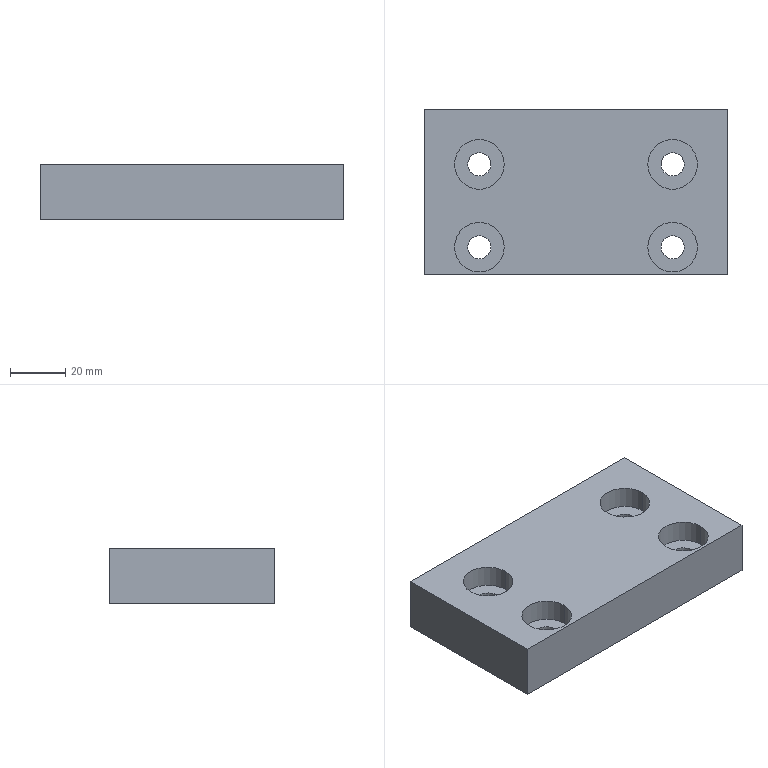Part | SolidWorks | features BaseBody 1 | 1 solid | 34 faces | box 110 x 60 x 20 mm | volume 118905 mm3 | cylinder 20 | plane 10 | cone 4 | commonest cylinder face diameters 8.4 x8 18 x8 10.2 x4
STEP:
#1=CARTESIAN_POINT('',(185.8,110.,-32.879));
#2=VERTEX_POINT('',#1);
#3=CARTESIAN_POINT('',(194.2,110.,-32.879));
#4=VERTEX_POINT('',#3);
#5=CARTESIAN_POINT('',(190.,110.,-32.879));
#6=DIRECTION('',(0.,0.,1.));
#7=DIRECTION('',(1.,0.,0.));
#8=AXIS2_PLACEMENT_3D('',#5,#6,#7);
#9=CIRCLE('',#8,4.2);
#10=EDGE_CURVE('',#2,#4,#9,.T.);
#11=ORIENTED_EDGE('',*,*,#10,.F.);
#12=CARTESIAN_POINT('',(185.8,110.,-20.879));
#13=VERTEX_POINT('',#12);
#14=CARTESIAN_POINT('',(185.8,110.,-12.879));
#15=DIRECTION('',(0.,0.,1.));
#16=VECTOR('',#15,1000.);
#17=LINE('',#14,#16);
#18=EDGE_CURVE('',#2,#13,#17,.T.);
#19=ORIENTED_EDGE('',*,*,#18,.T.);
#20=CARTESIAN_POINT('',(194.2,110.,-20.879));
#21=VERTEX_POINT('',#20);
#22=CARTESIAN_POINT('',(190.,110.,-20.879));
#23=DIRECTION('',(0.,0.,-1.));
#24=DIRECTION('',(1.,0.,0.));
#25=AXIS2_PLACEMENT_3D('',#22,#23,#24);
#26=CIRCLE('',#25,4.2);
#27=EDGE_CURVE('',#21,#13,#26,.T.);
#28=ORIENTED_EDGE('',*,*,#27,.F.);
#29=CARTESIAN_POINT('',(194.2,110.,-12.879));
#30=DIRECTION('',(0.,0.,1.));
#31=VECTOR('',#30,1000.);
#32=LINE('',#29,#31);
#33=EDGE_CURVE('',#4,#21,#32,.T.);
#34=ORIENTED_EDGE('',*,*,#33,.F.);
#35=EDGE_LOOP('',(#11,#19,#28,#34));
#36=FACE_OUTER_BOUND('',#35,.T.);
#37=CARTESIAN_POINT('',(190.,110.,-12.879));
#38=DIRECTION('',(0.,0.,1.));
#39=DIRECTION('',(1.,0.,0.));
#40=AXIS2_PLACEMENT_3D('',#37,#38,#39);
#41=CYLINDRICAL_SURFACE('',#40,4.2);
#42=ADVANCED_FACE('',(#36),#41,.F.);
#43=CARTESIAN_POINT('',(185.8,80.,-32.879));
#44=VERTEX_POINT('',#43);
#45=CARTESIAN_POINT('',(194.2,80.,-32.879));
#46=VERTEX_POINT('',#45);
#47=CARTESIAN_POINT('',(190.,80.,-32.879));
#48=DIRECTION('',(0.,0.,1.));
#49=DIRECTION('',(1.,0.,0.));
#50=AXIS2_PLACEMENT_3D('',#47,#48,#49);
#51=CIRCLE('',#50,4.2);
#52=EDGE_CURVE('',#44,#46,#51,.T.);
#53=ORIENTED_EDGE('',*,*,#52,.F.);
#54=CARTESIAN_POINT('',(185.8,80.,-20.879));
#55=VERTEX_POINT('',#54);
#56=CARTESIAN_POINT('',(185.8,80.,-12.879));
#57=DIRECTION('',(0.,0.,1.));
#58=VECTOR('',#57,1000.);
#59=LINE('',#56,#58);
#60=EDGE_CURVE('',#44,#55,#59,.T.);
#61=ORIENTED_EDGE('',*,*,#60,.T.);
#62=CARTESIAN_POINT('',(194.2,80.,-20.879));
#63=VERTEX_POINT('',#62);
#64=CARTESIAN_POINT('',(190.,80.,-20.879));
#65=DIRECTION('',(0.,0.,-1.));
#66=DIRECTION('',(1.,0.,0.));
#67=AXIS2_PLACEMENT_3D('',#64,#65,#66);
#68=CIRCLE('',#67,4.2);
#69=EDGE_CURVE('',#63,#55,#68,.T.);
#70=ORIENTED_EDGE('',*,*,#69,.F.);
#71=CARTESIAN_POINT('',(194.2,80.,-12.879));
#72=DIRECTION('',(0.,0.,1.));
#73=VECTOR('',#72,1000.);
#74=LINE('',#71,#73);
#75=EDGE_CURVE('',#46,#63,#74,.T.);
#76=ORIENTED_EDGE('',*,*,#75,.F.);
#77=EDGE_LOOP('',(#53,#61,#70,#76));
#78=FACE_OUTER_BOUND('',#77,.T.);
#79=CARTESIAN_POINT('',(190.,80.,-12.879));
#80=DIRECTION('',(0.,0.,1.));
#81=DIRECTION('',(1.,0.,0.));
#82=AXIS2_PLACEMENT_3D('',#79,#80,#81);
#83=CYLINDRICAL_SURFACE('',#82,4.2);
#84=ADVANCED_FACE('',(#78),#83,.F.);
#85=CARTESIAN_POINT('',(255.8,80.,-32.879));
#86=VERTEX_POINT('',#85);
#87=CARTESIAN_POINT('',(264.2,80.,-32.879));
#88=VERTEX_POINT('',#87);
#89=CARTESIAN_POINT('',(260.,80.,-32.879));
#90=DIRECTION('',(0.,0.,1.));
#91=DIRECTION('',(1.,0.,0.));
#92=AXIS2_PLACEMENT_3D('',#89,#90,#91);
#93=CIRCLE('',#92,4.2);
#94=EDGE_CURVE('',#86,#88,#93,.T.);
#95=ORIENTED_EDGE('',*,*,#94,.F.);
#96=CARTESIAN_POINT('',(255.8,80.,-20.879));
#97=VERTEX_POINT('',#96);
#98=CARTESIAN_POINT('',(255.8,80.,-12.879));
#99=DIRECTION('',(0.,0.,1.));
#100=VECTOR('',#99,1000.);
#101=LINE('',#98,#100);
#102=EDGE_CURVE('',#86,#97,#101,.T.);
#103=ORIENTED_EDGE('',*,*,#102,.T.);
#104=CARTESIAN_POINT('',(264.2,80.,-20.879));
#105=VERTEX_POINT('',#104);
#106=CARTESIAN_POINT('',(260.,80.,-20.879));
#107=DIRECTION('',(0.,0.,-1.));
#108=DIRECTION('',(1.,0.,0.));
#109=AXIS2_PLACEMENT_3D('',#106,#107,#108);
#110=CIRCLE('',#109,4.2);
#111=EDGE_CURVE('',#105,#97,#110,.T.);
#112=ORIENTED_EDGE('',*,*,#111,.F.);
#113=CARTESIAN_POINT('',(264.2,80.,-12.879));
#114=DIRECTION('',(0.,0.,1.));
#115=VECTOR('',#114,1000.);
#116=LINE('',#113,#115);
#117=EDGE_CURVE('',#88,#105,#116,.T.);
#118=ORIENTED_EDGE('',*,*,#117,.F.);
#119=EDGE_LOOP('',(#95,#103,#112,#118));
#120=FACE_OUTER_BOUND('',#119,.T.);
#121=CARTESIAN_POINT('',(260.,80.,-12.879));
#122=DIRECTION('',(0.,0.,1.));
#123=DIRECTION('',(1.,0.,0.));
#124=AXIS2_PLACEMENT_3D('',#121,#122,#123);
#125=CYLINDRICAL_SURFACE('',#124,4.2);
#126=ADVANCED_FACE('',(#120),#125,.F.);
#127=CARTESIAN_POINT('',(255.8,110.,-32.879));
#128=VERTEX_POINT('',#127);
#129=CARTESIAN_POINT('',(264.2,110.,-32.879));
#130=VERTEX_POINT('',#129);
#131=CARTESIAN_POINT('',(260.,110.,-32.879));
#132=DIRECTION('',(0.,0.,1.));
#133=DIRECTION('',(1.,0.,0.));
#134=AXIS2_PLACEMENT_3D('',#131,#132,#133);
#135=CIRCLE('',#134,4.2);
#136=EDGE_CURVE('',#128,#130,#135,.T.);
#137=ORIENTED_EDGE('',*,*,#136,.F.);
#138=CARTESIAN_POINT('',(255.8,110.,-20.879));
#139=VERTEX_POINT('',#138);
#140=CARTESIAN_POINT('',(255.8,110.,-12.879));
#141=DIRECTION('',(0.,0.,1.));
#142=VECTOR('',#141,1000.);
#143=LINE('',#140,#142);
#144=EDGE_CURVE('',#128,#139,#143,.T.);
#145=ORIENTED_EDGE('',*,*,#144,.T.);
#146=CARTESIAN_POINT('',(264.2,110.,-20.879));
#147=VERTEX_POINT('',#146);
#148=CARTESIAN_POINT('',(260.,110.,-20.879));
#149=DIRECTION('',(0.,0.,-1.));
#150=DIRECTION('',(1.,0.,0.));
#151=AXIS2_PLACEMENT_3D('',#148,#149,#150);
#152=CIRCLE('',#151,4.2);
#153=EDGE_CURVE('',#147,#139,#152,.T.);
#154=ORIENTED_EDGE('',*,*,#153,.F.);
#155=CARTESIAN_POINT('',(264.2,110.,-12.879));
#156=DIRECTION('',(0.,0.,1.));
#157=VECTOR('',#156,1000.);
#158=LINE('',#155,#157);
#159=EDGE_CURVE('',#130,#147,#158,.T.);
#160=ORIENTED_EDGE('',*,*,#159,.F.);
#161=EDGE_LOOP('',(#137,#145,#154,#160));
#162=FACE_OUTER_BOUND('',#161,.T.);
#163=CARTESIAN_POINT('',(260.,110.,-12.879));
#164=DIRECTION('',(0.,0.,1.));
#165=DIRECTION('',(1.,0.,0.));
#166=AXIS2_PLACEMENT_3D('',#163,#164,#165);
#167=CYLINDRICAL_SURFACE('',#166,4.2);
#168=ADVANCED_FACE('',(#162),#167,.F.);
#169=CARTESIAN_POINT('',(272.,117.,-27.979));
#170=VERTEX_POINT('',#169);
#171=CARTESIAN_POINT('',(272.,117.,-17.779));
#172=VERTEX_POINT('',#171);
#173=CARTESIAN_POINT('',(272.,117.,-22.879));
#174=DIRECTION('',(0.,1.,0.));
#175=DIRECTION('',(0.,0.,1.));
#176=AXIS2_PLACEMENT_3D('',#173,#174,#175);
#177=CIRCLE('',#176,5.1);
#178=EDGE_CURVE('',#170,#172,#177,.T.);
#179=ORIENTED_EDGE('',*,*,#178,.F.);
#180=CARTESIAN_POINT('',(272.,130.,-27.979));
#181=VERTEX_POINT('',#180);
#182=CARTESIAN_POINT('',(272.,130.,-27.979));
#183=DIRECTION('',(0.,1.,0.));
#184=VECTOR('',#183,1000.);
#185=LINE('',#182,#184);
#186=EDGE_CURVE('',#170,#181,#185,.T.);
#187=ORIENTED_EDGE('',*,*,#186,.T.);
#188=CARTESIAN_POINT('',(272.,130.,-17.779));
#189=VERTEX_POINT('',#188);
#190=CARTESIAN_POINT('',(272.,130.,-22.879));
#191=DIRECTION('',(0.,1.,0.));
#192=DIRECTION('',(0.,0.,1.));
#193=AXIS2_PLACEMENT_3D('',#190,#191,#192);
#194=CIRCLE('',#193,5.1);
#195=EDGE_CURVE('',#181,#189,#194,.T.);
#196=ORIENTED_EDGE('',*,*,#195,.T.);
#197=CARTESIAN_POINT('',(272.,130.,-17.779));
#198=DIRECTION('',(0.,1.,0.));
#199=VECTOR('',#198,1000.);
#200=LINE('',#197,#199);
#201=EDGE_CURVE('',#172,#189,#200,.T.);
#202=ORIENTED_EDGE('',*,*,#201,.F.);
#203=EDGE_LOOP('',(#179,#187,#196,#202));
#204=FACE_OUTER_BOUND('',#203,.T.);
#205=CARTESIAN_POINT('',(272.,130.,-22.879));
#206=DIRECTION('',(0.,1.,0.));
#207=DIRECTION('',(0.,0.,1.));
#208=AXIS2_PLACEMENT_3D('',#205,#206,#207);
#209=CYLINDRICAL_SURFACE('',#208,5.1);
#210=ADVANCED_FACE('',(#204),#209,.F.);
#211=CARTESIAN_POINT('',(178.,117.,-27.979));
#212=VERTEX_POINT('',#211);
#213=CARTESIAN_POINT('',(178.,117.,-17.779));
#214=VERTEX_POINT('',#213);
#215=CARTESIAN_POINT('',(178.,117.,-22.879));
#216=DIRECTION('',(0.,1.,0.));
#217=DIRECTION('',(0.,0.,1.));
#218=AXIS2_PLACEMENT_3D('',#215,#216,#217);
#219=CIRCLE('',#218,5.1);
#220=EDGE_CURVE('',#212,#214,#219,.T.);
#221=ORIENTED_EDGE('',*,*,#220,.F.);
#222=CARTESIAN_POINT('',(178.,130.,-27.979));
#223=VERTEX_POINT('',#222);
#224=CARTESIAN_POINT('',(178.,130.,-27.979));
#225=DIRECTION('',(0.,1.,0.));
#226=VECTOR('',#225,1000.);
#227=LINE('',#224,#226);
#228=EDGE_CURVE('',#212,#223,#227,.T.);
#229=ORIENTED_EDGE('',*,*,#228,.T.);
#230=CARTESIAN_POINT('',(178.,130.,-17.779));
#231=VERTEX_POINT('',#230);
#232=CARTESIAN_POINT('',(178.,130.,-22.879));
#233=DIRECTION('',(0.,1.,0.));
#234=DIRECTION('',(0.,0.,1.));
#235=AXIS2_PLACEMENT_3D('',#232,#233,#234);
#236=CIRCLE('',#235,5.1);
#237=EDGE_CURVE('',#223,#231,#236,.T.);
#238=ORIENTED_EDGE('',*,*,#237,.T.);
#239=CARTESIAN_POINT('',(178.,130.,-17.779));
#240=DIRECTION('',(0.,1.,0.));
#241=VECTOR('',#240,1000.);
#242=LINE('',#239,#241);
#243=EDGE_CURVE('',#214,#231,#242,.T.);
#244=ORIENTED_EDGE('',*,*,#243,.F.);
#245=EDGE_LOOP('',(#221,#229,#238,#244));
#246=FACE_OUTER_BOUND('',#245,.T.);
#247=CARTESIAN_POINT('',(178.,130.,-22.879));
#248=DIRECTION('',(0.,1.,0.));
#249=DIRECTION('',(0.,0.,1.));
#250=AXIS2_PLACEMENT_3D('',#247,#248,#249);
#251=CYLINDRICAL_SURFACE('',#250,5.1);
#252=ADVANCED_FACE('',(#246),#251,.F.);
#253=CARTESIAN_POINT('',(199.,110.,-20.879));
#254=VERTEX_POINT('',#253);
#255=CARTESIAN_POINT('',(181.,110.,-20.879));
#256=VERTEX_POINT('',#255);
#257=CARTESIAN_POINT('',(190.,110.,-20.879));
#258=DIRECTION('',(0.,0.,-1.));
#259=DIRECTION('',(1.,0.,0.));
#260=AXIS2_PLACEMENT_3D('',#257,#258,#259);
#261=CIRCLE('',#260,9.);
#262=EDGE_CURVE('',#254,#256,#261,.T.);
#263=ORIENTED_EDGE('',*,*,#262,.T.);
#264=CARTESIAN_POINT('',(181.,110.,-12.879));
#265=VERTEX_POINT('',#264);
#266=CARTESIAN_POINT('',(181.,110.,-12.879));
#267=DIRECTION('',(0.,0.,1.));
#268=VECTOR('',#267,1000.);
#269=LINE('',#266,#268);
#270=EDGE_CURVE('',#256,#265,#269,.T.);
#271=ORIENTED_EDGE('',*,*,#270,.T.);
#272=CARTESIAN_POINT('',(199.,110.,-12.879));
#273=VERTEX_POINT('',#272);
#274=CARTESIAN_POINT('',(190.,110.,-12.879));
#275=DIRECTION('',(0.,0.,1.));
#276=DIRECTION('',(1.,0.,0.));
#277=AXIS2_PLACEMENT_3D('',#274,#275,#276);
#278=CIRCLE('',#277,9.);
#279=EDGE_CURVE('',#265,#273,#278,.T.);
#280=ORIENTED_EDGE('',*,*,#279,.T.);
#281=CARTESIAN_POINT('',(199.,110.,-12.879));
#282=DIRECTION('',(0.,0.,1.));
#283=VECTOR('',#282,1000.);
#284=LINE('',#281,#283);
#285=EDGE_CURVE('',#254,#273,#284,.T.);
#286=ORIENTED_EDGE('',*,*,#285,.F.);
#287=EDGE_LOOP('',(#263,#271,#280,#286));
#288=FACE_OUTER_BOUND('',#287,.T.);
#289=CARTESIAN_POINT('',(190.,110.,-12.879));
#290=DIRECTION('',(0.,0.,1.));
#291=DIRECTION('',(1.,0.,0.));
#292=AXIS2_PLACEMENT_3D('',#289,#290,#291);
#293=CYLINDRICAL_SURFACE('',#292,9.);
#294=ADVANCED_FACE('',(#288),#293,.F.);
#295=CARTESIAN_POINT('',(199.,80.,-20.879));
#296=VERTEX_POINT('',#295);
#297=CARTESIAN_POINT('',(181.,80.,-20.879));
#298=VERTEX_POINT('',#297);
#299=CARTESIAN_POINT('',(190.,80.,-20.879));
#300=DIRECTION('',(0.,0.,-1.));
#301=DIRECTION('',(1.,0.,0.));
#302=AXIS2_PLACEMENT_3D('',#299,#300,#301);
#303=CIRCLE('',#302,9.);
#304=EDGE_CURVE('',#296,#298,#303,.T.);
#305=ORIENTED_EDGE('',*,*,#304,.T.);
#306=CARTESIAN_POINT('',(181.,80.,-12.879));
#307=VERTEX_POINT('',#306);
#308=CARTESIAN_POINT('',(181.,80.,-12.879));
#309=DIRECTION('',(0.,0.,1.));
#310=VECTOR('',#309,1000.);
#311=LINE('',#308,#310);
#312=EDGE_CURVE('',#298,#307,#311,.T.);
#313=ORIENTED_EDGE('',*,*,#312,.T.);
#314=CARTESIAN_POINT('',(199.,80.,-12.879));
#315=VERTEX_POINT('',#314);
#316=CARTESIAN_POINT('',(190.,80.,-12.879));
#317=DIRECTION('',(0.,0.,1.));
#318=DIRECTION('',(1.,0.,0.));
#319=AXIS2_PLACEMENT_3D('',#316,#317,#318);
#320=CIRCLE('',#319,9.);
#321=EDGE_CURVE('',#307,#315,#320,.T.);
#322=ORIENTED_EDGE('',*,*,#321,.T.);
#323=CARTESIAN_POINT('',(199.,80.,-12.879));
#324=DIRECTION('',(0.,0.,1.));
#325=VECTOR('',#324,1000.);
#326=LINE('',#323,#325);
#327=EDGE_CURVE('',#296,#315,#326,.T.);
#328=ORIENTED_EDGE('',*,*,#327,.F.);
#329=EDGE_LOOP('',(#305,#313,#322,#328));
#330=FACE_OUTER_BOUND('',#329,.T.);
#331=CARTESIAN_POINT('',(190.,80.,-12.879));
#332=DIRECTION('',(0.,0.,1.));
#333=DIRECTION('',(1.,0.,0.));
#334=AXIS2_PLACEMENT_3D('',#331,#332,#333);
#335=CYLINDRICAL_SURFACE('',#334,9.);
#336=ADVANCED_FACE('',(#330),#335,.F.);
#337=CARTESIAN_POINT('',(269.,80.,-20.879));
#338=VERTEX_POINT('',#337);
#339=CARTESIAN_POINT('',(251.,80.,-20.879));
#340=VERTEX_POINT('',#339);
#341=CARTESIAN_POINT('',(260.,80.,-20.879));
#342=DIRECTION('',(0.,0.,-1.));
#343=DIRECTION('',(1.,0.,0.));
#344=AXIS2_PLACEMENT_3D('',#341,#342,#343);
#345=CIRCLE('',#344,9.);
#346=EDGE_CURVE('',#338,#340,#345,.T.);
#347=ORIENTED_EDGE('',*,*,#346,.T.);
#348=CARTESIAN_POINT('',(251.,80.,-12.879));
#349=VERTEX_POINT('',#348);
#350=CARTESIAN_POINT('',(251.,80.,-12.879));
#351=DIRECTION('',(0.,0.,1.));
#352=VECTOR('',#351,1000.);
#353=LINE('',#350,#352);
#354=EDGE_CURVE('',#340,#349,#353,.T.);
#355=ORIENTED_EDGE('',*,*,#354,.T.);
#356=CARTESIAN_POINT('',(269.,80.,-12.879));
#357=VERTEX_POINT('',#356);
#358=CARTESIAN_POINT('',(260.,80.,-12.879));
#359=DIRECTION('',(0.,0.,1.));
#360=DIRECTION('',(1.,0.,0.));
#361=AXIS2_PLACEMENT_3D('',#358,#359,#360);
#362=CIRCLE('',#361,9.);
#363=EDGE_CURVE('',#349,#357,#362,.T.);
#364=ORIENTED_EDGE('',*,*,#363,.T.);
#365=CARTESIAN_POINT('',(269.,80.,-12.879));
#366=DIRECTION('',(0.,0.,1.));
#367=VECTOR('',#366,1000.);
#368=LINE('',#365,#367);
#369=EDGE_CURVE('',#338,#357,#368,.T.);
#370=ORIENTED_EDGE('',*,*,#369,.F.);
#371=EDGE_LOOP('',(#347,#355,#364,#370));
#372=FACE_OUTER_BOUND('',#371,.T.);
#373=CARTESIAN_POINT('',(260.,80.,-12.879));
#374=DIRECTION('',(0.,0.,1.));
#375=DIRECTION('',(1.,0.,0.));
#376=AXIS2_PLACEMENT_3D('',#373,#374,#375);
#377=CYLINDRICAL_SURFACE('',#376,9.);
#378=ADVANCED_FACE('',(#372),#377,.F.);
#379=CARTESIAN_POINT('',(269.,110.,-20.879));
#380=VERTEX_POINT('',#379);
#381=CARTESIAN_POINT('',(251.,110.,-20.879));
#382=VERTEX_POINT('',#381);
#383=CARTESIAN_POINT('',(260.,110.,-20.879));
#384=DIRECTION('',(0.,0.,-1.));
#385=DIRECTION('',(1.,0.,0.));
#386=AXIS2_PLACEMENT_3D('',#383,#384,#385);
#387=CIRCLE('',#386,9.);
#388=EDGE_CURVE('',#380,#382,#387,.T.);
#389=ORIENTED_EDGE('',*,*,#388,.T.);
#390=CARTESIAN_POINT('',(251.,110.,-12.879));
#391=VERTEX_POINT('',#390);
#392=CARTESIAN_POINT('',(251.,110.,-12.879));
#393=DIRECTION('',(0.,0.,1.));
#394=VECTOR('',#393,1000.);
#395=LINE('',#392,#394);
#396=EDGE_CURVE('',#382,#391,#395,.T.);
#397=ORIENTED_EDGE('',*,*,#396,.T.);
#398=CARTESIAN_POINT('',(269.,110.,-12.879));
#399=VERTEX_POINT('',#398);
#400=CARTESIAN_POINT('',(260.,110.,-12.879));
#401=DIRECTION('',(0.,0.,1.));
#402=DIRECTION('',(1.,0.,0.));
#403=AXIS2_PLACEMENT_3D('',#400,#401,#402);
#404=CIRCLE('',#403,9.);
#405=EDGE_CURVE('',#391,#399,#404,.T.);
#406=ORIENTED_EDGE('',*,*,#405,.T.);
#407=CARTESIAN_POINT('',(269.,110.,-12.879));
#408=DIRECTION('',(0.,0.,1.));
#409=VECTOR('',#408,1000.);
#410=LINE('',#407,#409);
#411=EDGE_CURVE('',#380,#399,#410,.T.);
#412=ORIENTED_EDGE('',*,*,#411,.F.);
#413=EDGE_LOOP('',(#389,#397,#406,#412));
#414=FACE_OUTER_BOUND('',#413,.T.);
#415=CARTESIAN_POINT('',(260.,110.,-12.879));
#416=DIRECTION('',(0.,0.,1.));
#417=DIRECTION('',(1.,0.,0.));
#418=AXIS2_PLACEMENT_3D('',#415,#416,#417);
#419=CYLINDRICAL_SURFACE('',#418,9.);
#420=ADVANCED_FACE('',(#414),#419,.F.);
#421=CARTESIAN_POINT('',(272.,113.936,-22.879));
#422=VERTEX_POINT('',#421);
#423=CARTESIAN_POINT('',(272.,117.,-17.779));
#424=DIRECTION('',(0.,0.515,0.8572));
#425=VECTOR('',#424,1000.);
#426=LINE('',#423,#425);
#427=EDGE_CURVE('',#422,#172,#426,.T.);
#428=ORIENTED_EDGE('',*,*,#427,.F.);
#429=CARTESIAN_POINT('',(272.,117.,-27.979));
#430=DIRECTION('',(0.,0.515,-0.8572));
#431=VECTOR('',#430,1000.);
#432=LINE('',#429,#431);
#433=EDGE_CURVE('',#422,#170,#432,.T.);
#434=ORIENTED_EDGE('',*,*,#433,.T.);
#435=ORIENTED_EDGE('',*,*,#178,.T.);
#436=EDGE_LOOP('',(#428,#434,#435));
#437=FACE_OUTER_BOUND('',#436,.T.);
#438=CARTESIAN_POINT('',(272.,117.,-22.879));
#439=DIRECTION('',(0.,1.,0.));
#440=DIRECTION('',(0.,0.,1.));
#441=AXIS2_PLACEMENT_3D('',#438,#439,#440);
#442=CONICAL_SURFACE('',#441,5.1,1.03);
#443=ADVANCED_FACE('',(#437),#442,.F.);
#444=CARTESIAN_POINT('',(178.,113.936,-22.879));
#445=VERTEX_POINT('',#444);
#446=CARTESIAN_POINT('',(178.,117.,-17.779));
#447=DIRECTION('',(0.,0.515,0.8572));
#448=VECTOR('',#447,1000.);
#449=LINE('',#446,#448);
#450=EDGE_CURVE('',#445,#214,#449,.T.);
#451=ORIENTED_EDGE('',*,*,#450,.F.);
#452=CARTESIAN_POINT('',(178.,117.,-27.979));
#453=DIRECTION('',(0.,0.515,-0.8572));
#454=VECTOR('',#453,1000.);
#455=LINE('',#452,#454);
#456=EDGE_CURVE('',#445,#212,#455,.T.);
#457=ORIENTED_EDGE('',*,*,#456,.T.);
#458=ORIENTED_EDGE('',*,*,#220,.T.);
#459=EDGE_LOOP('',(#451,#457,#458));
#460=FACE_OUTER_BOUND('',#459,.T.);
#461=CARTESIAN_POINT('',(178.,117.,-22.879));
#462=DIRECTION('',(0.,1.,0.));
#463=DIRECTION('',(0.,0.,1.));
#464=AXIS2_PLACEMENT_3D('',#461,#462,#463);
#465=CONICAL_SURFACE('',#464,5.1,1.03);
#466=ADVANCED_FACE('',(#460),#465,.F.);
#467=CARTESIAN_POINT('',(170.,70.,-32.879));
#468=VERTEX_POINT('',#467);
#469=CARTESIAN_POINT('',(170.,130.,-32.879));
#470=VERTEX_POINT('',#469);
#471=CARTESIAN_POINT('',(170.,100.,-32.879));
#472=DIRECTION('',(0.,1.,0.));
#473=VECTOR('',#472,1000.);
#474=LINE('',#471,#473);
#475=EDGE_CURVE('',#468,#470,#474,.T.);
#476=ORIENTED_EDGE('',*,*,#475,.T.);
#477=CARTESIAN_POINT('',(280.,130.,-32.879));
#478=VERTEX_POINT('',#477);
#479=CARTESIAN_POINT('',(225.,130.,-32.879));
#480=DIRECTION('',(1.,0.,0.));
#481=VECTOR('',#480,1000.);
#482=LINE('',#479,#481);
#483=EDGE_CURVE('',#470,#478,#482,.T.);
#484=ORIENTED_EDGE('',*,*,#483,.T.);
#485=CARTESIAN_POINT('',(280.,70.,-32.879));
#486=VERTEX_POINT('',#485);
#487=CARTESIAN_POINT('',(280.,100.,-32.879));
#488=DIRECTION('',(0.,-1.,0.));
#489=VECTOR('',#488,1000.);
#490=LINE('',#487,#489);
#491=EDGE_CURVE('',#478,#486,#490,.T.);
#492=ORIENTED_EDGE('',*,*,#491,.T.);
#493=CARTESIAN_POINT('',(225.,70.,-32.879));
#494=DIRECTION('',(-1.,0.,0.));
#495=VECTOR('',#494,1000.);
#496=LINE('',#493,#495);
#497=EDGE_CURVE('',#486,#468,#496,.T.);
#498=ORIENTED_EDGE('',*,*,#497,.T.);
#499=EDGE_LOOP('',(#476,#484,#492,#498));
#500=FACE_OUTER_BOUND('',#499,.T.);
#501=CARTESIAN_POINT('',(190.,110.,-32.879));
#502=DIRECTION('',(0.,0.,1.));
#503=DIRECTION('',(1.,0.,0.));
#504=AXIS2_PLACEMENT_3D('',#501,#502,#503);
#505=CIRCLE('',#504,4.2);
#506=EDGE_CURVE('',#4,#2,#505,.T.);
#507=ORIENTED_EDGE('',*,*,#506,.T.);
#508=ORIENTED_EDGE('',*,*,#10,.T.);
#509=EDGE_LOOP('',(#507,#508));
#510=FACE_BOUND('',#509,.T.);
#511=CARTESIAN_POINT('',(190.,80.,-32.879));
#512=DIRECTION('',(0.,0.,1.));
#513=DIRECTION('',(1.,0.,0.));
#514=AXIS2_PLACEMENT_3D('',#511,#512,#513);
#515=CIRCLE('',#514,4.2);
#516=EDGE_CURVE('',#46,#44,#515,.T.);
#517=ORIENTED_EDGE('',*,*,#516,.T.);
#518=ORIENTED_EDGE('',*,*,#52,.T.);
#519=EDGE_LOOP('',(#517,#518));
#520=FACE_BOUND('',#519,.T.);
#521=CARTESIAN_POINT('',(260.,80.,-32.879));
#522=DIRECTION('',(0.,0.,1.));
#523=DIRECTION('',(1.,0.,0.));
#524=AXIS2_PLACEMENT_3D('',#521,#522,#523);
#525=CIRCLE('',#524,4.2);
#526=EDGE_CURVE('',#88,#86,#525,.T.);
#527=ORIENTED_EDGE('',*,*,#526,.T.);
#528=ORIENTED_EDGE('',*,*,#94,.T.);
#529=EDGE_LOOP('',(#527,#528));
#530=FACE_BOUND('',#529,.T.);
#531=CARTESIAN_POINT('',(260.,110.,-32.879));
#532=DIRECTION('',(0.,0.,1.));
#533=DIRECTION('',(1.,0.,0.));
#534=AXIS2_PLACEMENT_3D('',#531,#532,#533);
#535=CIRCLE('',#534,4.2);
#536=EDGE_CURVE('',#130,#128,#535,.T.);
#537=ORIENTED_EDGE('',*,*,#536,.T.);
#538=ORIENTED_EDGE('',*,*,#136,.T.);
#539=EDGE_LOOP('',(#537,#538));
#540=FACE_BOUND('',#539,.T.);
#541=CARTESIAN_POINT('',(225.,100.,-32.879));
#542=DIRECTION('',(0.,0.,-1.));
#543=DIRECTION('',(-1.,0.,0.));
#544=AXIS2_PLACEMENT_3D('',#541,#542,#543);
#545=PLANE('',#544);
#546=ADVANCED_FACE('',(#500,#510,#520,#530,#540),#545,.T.);
#547=CARTESIAN_POINT('',(170.,130.,-12.879));
#548=VERTEX_POINT('',#547);
#549=CARTESIAN_POINT('',(170.,130.,-12.879));
#550=DIRECTION('',(0.,0.,-1.));
#551=VECTOR('',#550,1000.);
#552=LINE('',#549,#551);
#553=EDGE_CURVE('',#548,#470,#552,.T.);
#554=ORIENTED_EDGE('',*,*,#553,.F.);
#555=CARTESIAN_POINT('',(280.,130.,-12.879));
#556=VERTEX_POINT('',#555);
#557=CARTESIAN_POINT('',(170.,130.,-12.879));
#558=DIRECTION('',(-1.,0.,0.));
#559=VECTOR('',#558,1000.);
#560=LINE('',#557,#559);
#561=EDGE_CURVE('',#556,#548,#560,.T.);
#562=ORIENTED_EDGE('',*,*,#561,.F.);
#563=CARTESIAN_POINT('',(280.,130.,-12.879));
#564=DIRECTION('',(0.,0.,1.));
#565=VECTOR('',#564,1000.);
#566=LINE('',#563,#565);
#567=EDGE_CURVE('',#478,#556,#566,.T.);
#568=ORIENTED_EDGE('',*,*,#567,.F.);
#569=ORIENTED_EDGE('',*,*,#483,.F.);
#570=EDGE_LOOP('',(#554,#562,#568,#569));
#571=FACE_OUTER_BOUND('',#570,.T.);
#572=CARTESIAN_POINT('',(272.,130.,-22.879));
#573=DIRECTION('',(0.,1.,0.));
#574=DIRECTION('',(0.,0.,1.));
#575=AXIS2_PLACEMENT_3D('',#572,#573,#574);
#576=CIRCLE('',#575,5.1);
#577=EDGE_CURVE('',#189,#181,#576,.T.);
#578=ORIENTED_EDGE('',*,*,#577,.F.);
#579=ORIENTED_EDGE('',*,*,#195,.F.);
#580=EDGE_LOOP('',(#578,#579));
#581=FACE_BOUND('',#580,.T.);
#582=CARTESIAN_POINT('',(178.,130.,-22.879));
#583=DIRECTION('',(0.,1.,0.));
#584=DIRECTION('',(0.,0.,1.));
#585=AXIS2_PLACEMENT_3D('',#582,#583,#584);
#586=CIRCLE('',#585,5.1);
#587=EDGE_CURVE('',#231,#223,#586,.T.);
#588=ORIENTED_EDGE('',*,*,#587,.F.);
#589=ORIENTED_EDGE('',*,*,#237,.F.);
#590=EDGE_LOOP('',(#588,#589));
#591=FACE_BOUND('',#590,.T.);
#592=CARTESIAN_POINT('',(170.,130.,-12.879));
#593=DIRECTION('',(0.,-1.,0.));
#594=DIRECTION('',(0.,0.,-1.));
#595=AXIS2_PLACEMENT_3D('',#592,#593,#594);
#596=PLANE('',#595);
#597=ADVANCED_FACE('',(#571,#581,#591),#596,.F.);
#598=CARTESIAN_POINT('',(170.,70.,-12.879));
#599=VERTEX_POINT('',#598);
#600=CARTESIAN_POINT('',(170.,70.,-12.879));
#601=DIRECTION('',(0.,0.,-1.));
#602=VECTOR('',#601,1000.);
#603=LINE('',#600,#602);
#604=EDGE_CURVE('',#599,#468,#603,.T.);
#605=ORIENTED_EDGE('',*,*,#604,.F.);
#606=CARTESIAN_POINT('',(170.,70.,-12.879));
#607=DIRECTION('',(0.,-1.,0.));
#608=VECTOR('',#607,1000.);
#609=LINE('',#606,#608);
#610=EDGE_CURVE('',#548,#599,#609,.T.);
#611=ORIENTED_EDGE('',*,*,#610,.F.);
#612=ORIENTED_EDGE('',*,*,#553,.T.);
#613=ORIENTED_EDGE('',*,*,#475,.F.);
#614=EDGE_LOOP('',(#605,#611,#612,#613));
#615=FACE_OUTER_BOUND('',#614,.T.);
#616=CARTESIAN_POINT('',(170.,70.,-12.879));
#617=DIRECTION('',(1.,0.,0.));
#618=DIRECTION('',(0.,0.,-1.));
#619=AXIS2_PLACEMENT_3D('',#616,#617,#618);
#620=PLANE('',#619);
#621=ADVANCED_FACE('',(#615),#620,.F.);
#622=CARTESIAN_POINT('',(280.,70.,-12.879));
#623=VERTEX_POINT('',#622);
#624=CARTESIAN_POINT('',(280.,70.,-12.879));
#625=DIRECTION('',(0.,0.,-1.));
#626=VECTOR('',#625,1000.);
#627=LINE('',#624,#626);
#628=EDGE_CURVE('',#623,#486,#627,.T.);
#629=ORIENTED_EDGE('',*,*,#628,.F.);
#630=CARTESIAN_POINT('',(170.,70.,-12.879));
#631=DIRECTION('',(1.,0.,0.));
#632=VECTOR('',#631,1000.);
#633=LINE('',#630,#632);
#634=EDGE_CURVE('',#599,#623,#633,.T.);
#635=ORIENTED_EDGE('',*,*,#634,.F.);
#636=ORIENTED_EDGE('',*,*,#604,.T.);
#637=ORIENTED_EDGE('',*,*,#497,.F.);
#638=EDGE_LOOP('',(#629,#635,#636,#637));
#639=FACE_OUTER_BOUND('',#638,.T.);
#640=CARTESIAN_POINT('',(170.,70.,-12.879));
#641=DIRECTION('',(0.,1.,0.));
#642=DIRECTION('',(0.,0.,1.));
#643=AXIS2_PLACEMENT_3D('',#640,#641,#642);
#644=PLANE('',#643);
#645=ADVANCED_FACE('',(#639),#644,.F.);
#646=ORIENTED_EDGE('',*,*,#567,.T.);
#647=CARTESIAN_POINT('',(280.,70.,-12.879));
#648=DIRECTION('',(0.,1.,0.));
#649=VECTOR('',#648,1000.);
#650=LINE('',#647,#649);
#651=EDGE_CURVE('',#623,#556,#650,.T.);
#652=ORIENTED_EDGE('',*,*,#651,.F.);
#653=ORIENTED_EDGE('',*,*,#628,.T.);
#654=ORIENTED_EDGE('',*,*,#491,.F.);
#655=EDGE_LOOP('',(#646,#652,#653,#654));
#656=FACE_OUTER_BOUND('',#655,.T.);
#657=CARTESIAN_POINT('',(280.,70.,-12.879));
#658=DIRECTION('',(-1.,0.,0.));
#659=DIRECTION('',(0.,0.,1.));
#660=AXIS2_PLACEMENT_3D('',#657,#658,#659);
#661=PLANE('',#660);
#662=ADVANCED_FACE('',(#656),#661,.F.);
#663=ORIENTED_EDGE('',*,*,#18,.F.);
#664=ORIENTED_EDGE('',*,*,#506,.F.);
#665=ORIENTED_EDGE('',*,*,#33,.T.);
#666=CARTESIAN_POINT('',(190.,110.,-20.879));
#667=DIRECTION('',(0.,0.,-1.));
#668=DIRECTION('',(1.,0.,0.));
#669=AXIS2_PLACEMENT_3D('',#666,#667,#668);
#670=CIRCLE('',#669,4.2);
#671=EDGE_CURVE('',#13,#21,#670,.T.);
#672=ORIENTED_EDGE('',*,*,#671,.F.);
#673=EDGE_LOOP('',(#663,#664,#665,#672));
#674=FACE_OUTER_BOUND('',#673,.T.);
#675=CARTESIAN_POINT('',(190.,110.,-12.879));
#676=DIRECTION('',(0.,0.,1.));
#677=DIRECTION('',(1.,0.,0.));
#678=AXIS2_PLACEMENT_3D('',#675,#676,#677);
#679=CYLINDRICAL_SURFACE('',#678,4.2);
#680=ADVANCED_FACE('',(#674),#679,.F.);
#681=ORIENTED_EDGE('',*,*,#60,.F.);
#682=ORIENTED_EDGE('',*,*,#516,.F.);
#683=ORIENTED_EDGE('',*,*,#75,.T.);
#684=CARTESIAN_POINT('',(190.,80.,-20.879));
#685=DIRECTION('',(0.,0.,-1.));
#686=DIRECTION('',(1.,0.,0.));
#687=AXIS2_PLACEMENT_3D('',#684,#685,#686);
#688=CIRCLE('',#687,4.2);
#689=EDGE_CURVE('',#55,#63,#688,.T.);
#690=ORIENTED_EDGE('',*,*,#689,.F.);
#691=EDGE_LOOP('',(#681,#682,#683,#690));
#692=FACE_OUTER_BOUND('',#691,.T.);
#693=CARTESIAN_POINT('',(190.,80.,-12.879));
#694=DIRECTION('',(0.,0.,1.));
#695=DIRECTION('',(1.,0.,0.));
#696=AXIS2_PLACEMENT_3D('',#693,#694,#695);
#697=CYLINDRICAL_SURFACE('',#696,4.2);
#698=ADVANCED_FACE('',(#692),#697,.F.);
#699=ORIENTED_EDGE('',*,*,#102,.F.);
#700=ORIENTED_EDGE('',*,*,#526,.F.);
#701=ORIENTED_EDGE('',*,*,#117,.T.);
#702=CARTESIAN_POINT('',(260.,80.,-20.879));
#703=DIRECTION('',(0.,0.,-1.));
#704=DIRECTION('',(1.,0.,0.));
#705=AXIS2_PLACEMENT_3D('',#702,#703,#704);
#706=CIRCLE('',#705,4.2);
#707=EDGE_CURVE('',#97,#105,#706,.T.);
#708=ORIENTED_EDGE('',*,*,#707,.F.);
#709=EDGE_LOOP('',(#699,#700,#701,#708));
#710=FACE_OUTER_BOUND('',#709,.T.);
#711=CARTESIAN_POINT('',(260.,80.,-12.879));
#712=DIRECTION('',(0.,0.,1.));
#713=DIRECTION('',(1.,0.,0.));
#714=AXIS2_PLACEMENT_3D('',#711,#712,#713);
#715=CYLINDRICAL_SURFACE('',#714,4.2);
#716=ADVANCED_FACE('',(#710),#715,.F.);
#717=ORIENTED_EDGE('',*,*,#144,.F.);
#718=ORIENTED_EDGE('',*,*,#536,.F.);
#719=ORIENTED_EDGE('',*,*,#159,.T.);
#720=CARTESIAN_POINT('',(260.,110.,-20.879));
#721=DIRECTION('',(0.,0.,-1.));
#722=DIRECTION('',(1.,0.,0.));
#723=AXIS2_PLACEMENT_3D('',#720,#721,#722);
#724=CIRCLE('',#723,4.2);
#725=EDGE_CURVE('',#139,#147,#724,.T.);
#726=ORIENTED_EDGE('',*,*,#725,.F.);
#727=EDGE_LOOP('',(#717,#718,#719,#726));
#728=FACE_OUTER_BOUND('',#727,.T.);
#729=CARTESIAN_POINT('',(260.,110.,-12.879));
#730=DIRECTION('',(0.,0.,1.));
#731=DIRECTION('',(1.,0.,0.));
#732=AXIS2_PLACEMENT_3D('',#729,#730,#731);
#733=CYLINDRICAL_SURFACE('',#732,4.2);
#734=ADVANCED_FACE('',(#728),#733,.F.);
#735=ORIENTED_EDGE('',*,*,#561,.T.);
#736=ORIENTED_EDGE('',*,*,#610,.T.);
#737=ORIENTED_EDGE('',*,*,#634,.T.);
#738=ORIENTED_EDGE('',*,*,#651,.T.);
#739=EDGE_LOOP('',(#735,#736,#737,#738));
#740=FACE_OUTER_BOUND('',#739,.T.);
#741=CARTESIAN_POINT('',(190.,110.,-12.879));
#742=DIRECTION('',(0.,0.,1.));
#743=DIRECTION('',(1.,0.,0.));
#744=AXIS2_PLACEMENT_3D('',#741,#742,#743);
#745=CIRCLE('',#744,9.);
#746=EDGE_CURVE('',#273,#265,#745,.T.);
#747=ORIENTED_EDGE('',*,*,#746,.F.);
#748=ORIENTED_EDGE('',*,*,#279,.F.);
#749=EDGE_LOOP('',(#747,#748));
#750=FACE_BOUND('',#749,.T.);
#751=CARTESIAN_POINT('',(190.,80.,-12.879));
#752=DIRECTION('',(0.,0.,1.));
#753=DIRECTION('',(1.,0.,0.));
#754=AXIS2_PLACEMENT_3D('',#751,#752,#753);
#755=CIRCLE('',#754,9.);
#756=EDGE_CURVE('',#315,#307,#755,.T.);
#757=ORIENTED_EDGE('',*,*,#756,.F.);
#758=ORIENTED_EDGE('',*,*,#321,.F.);
#759=EDGE_LOOP('',(#757,#758));
#760=FACE_BOUND('',#759,.T.);
#761=CARTESIAN_POINT('',(260.,80.,-12.879));
#762=DIRECTION('',(0.,0.,1.));
#763=DIRECTION('',(1.,0.,0.));
#764=AXIS2_PLACEMENT_3D('',#761,#762,#763);
#765=CIRCLE('',#764,9.);
#766=EDGE_CURVE('',#357,#349,#765,.T.);
#767=ORIENTED_EDGE('',*,*,#766,.F.);
#768=ORIENTED_EDGE('',*,*,#363,.F.);
#769=EDGE_LOOP('',(#767,#768));
#770=FACE_BOUND('',#769,.T.);
#771=CARTESIAN_POINT('',(260.,110.,-12.879));
#772=DIRECTION('',(0.,0.,1.));
#773=DIRECTION('',(1.,0.,0.));
#774=AXIS2_PLACEMENT_3D('',#771,#772,#773);
#775=CIRCLE('',#774,9.);
#776=EDGE_CURVE('',#399,#391,#775,.T.);
#777=ORIENTED_EDGE('',*,*,#776,.F.);
#778=ORIENTED_EDGE('',*,*,#405,.F.);
#779=EDGE_LOOP('',(#777,#778));
#780=FACE_BOUND('',#779,.T.);
#781=CARTESIAN_POINT('',(225.,100.,-12.879));
#782=DIRECTION('',(0.,0.,-1.));
#783=DIRECTION('',(-1.,0.,0.));
#784=AXIS2_PLACEMENT_3D('',#781,#782,#783);
#785=PLANE('',#784);
#786=ADVANCED_FACE('',(#740,#750,#760,#770,#780),#785,.F.);
#787=ORIENTED_EDGE('',*,*,#186,.F.);
#788=CARTESIAN_POINT('',(272.,117.,-22.879));
#789=DIRECTION('',(0.,1.,0.));
#790=DIRECTION('',(0.,0.,1.));
#791=AXIS2_PLACEMENT_3D('',#788,#789,#790);
#792=CIRCLE('',#791,5.1);
#793=EDGE_CURVE('',#172,#170,#792,.T.);
#794=ORIENTED_EDGE('',*,*,#793,.F.);
#795=ORIENTED_EDGE('',*,*,#201,.T.);
#796=ORIENTED_EDGE('',*,*,#577,.T.);
#797=EDGE_LOOP('',(#787,#794,#795,#796));
#798=FACE_OUTER_BOUND('',#797,.T.);
#799=CARTESIAN_POINT('',(272.,130.,-22.879));
#800=DIRECTION('',(0.,1.,0.));
#801=DIRECTION('',(0.,0.,1.));
#802=AXIS2_PLACEMENT_3D('',#799,#800,#801);
#803=CYLINDRICAL_SURFACE('',#802,5.1);
#804=ADVANCED_FACE('',(#798),#803,.F.);
#805=ORIENTED_EDGE('',*,*,#228,.F.);
#806=CARTESIAN_POINT('',(178.,117.,-22.879));
#807=DIRECTION('',(0.,1.,0.));
#808=DIRECTION('',(0.,0.,1.));
#809=AXIS2_PLACEMENT_3D('',#806,#807,#808);
#810=CIRCLE('',#809,5.1);
#811=EDGE_CURVE('',#214,#212,#810,.T.);
#812=ORIENTED_EDGE('',*,*,#811,.F.);
#813=ORIENTED_EDGE('',*,*,#243,.T.);
#814=ORIENTED_EDGE('',*,*,#587,.T.);
#815=EDGE_LOOP('',(#805,#812,#813,#814));
#816=FACE_OUTER_BOUND('',#815,.T.);
#817=CARTESIAN_POINT('',(178.,130.,-22.879));
#818=DIRECTION('',(0.,1.,0.));
#819=DIRECTION('',(0.,0.,1.));
#820=AXIS2_PLACEMENT_3D('',#817,#818,#819);
#821=CYLINDRICAL_SURFACE('',#820,5.1);
#822=ADVANCED_FACE('',(#816),#821,.F.);
#823=ORIENTED_EDGE('',*,*,#262,.F.);
#824=CARTESIAN_POINT('',(190.,110.,-20.879));
#825=DIRECTION('',(0.,0.,-1.));
#826=DIRECTION('',(1.,0.,0.));
#827=AXIS2_PLACEMENT_3D('',#824,#825,#826);
#828=CIRCLE('',#827,9.);
#829=EDGE_CURVE('',#256,#254,#828,.T.);
#830=ORIENTED_EDGE('',*,*,#829,.F.);
#831=EDGE_LOOP('',(#823,#830));
#832=FACE_OUTER_BOUND('',#831,.T.);
#833=ORIENTED_EDGE('',*,*,#27,.T.);
#834=ORIENTED_EDGE('',*,*,#671,.T.);
#835=EDGE_LOOP('',(#833,#834));
#836=FACE_BOUND('',#835,.T.);
#837=CARTESIAN_POINT('',(194.2,110.,-20.879));
#838=DIRECTION('',(0.,0.,-1.));
#839=DIRECTION('',(-1.,0.,0.));
#840=AXIS2_PLACEMENT_3D('',#837,#838,#839);
#841=PLANE('',#840);
#842=ADVANCED_FACE('',(#832,#836),#841,.F.);
#843=ORIENTED_EDGE('',*,*,#304,.F.);
#844=CARTESIAN_POINT('',(190.,80.,-20.879));
#845=DIRECTION('',(0.,0.,-1.));
#846=DIRECTION('',(1.,0.,0.));
#847=AXIS2_PLACEMENT_3D('',#844,#845,#846);
#848=CIRCLE('',#847,9.);
#849=EDGE_CURVE('',#298,#296,#848,.T.);
#850=ORIENTED_EDGE('',*,*,#849,.F.);
#851=EDGE_LOOP('',(#843,#850));
#852=FACE_OUTER_BOUND('',#851,.T.);
#853=ORIENTED_EDGE('',*,*,#69,.T.);
#854=ORIENTED_EDGE('',*,*,#689,.T.);
#855=EDGE_LOOP('',(#853,#854));
#856=FACE_BOUND('',#855,.T.);
#857=CARTESIAN_POINT('',(194.2,80.,-20.879));
#858=DIRECTION('',(0.,0.,-1.));
#859=DIRECTION('',(-1.,0.,0.));
#860=AXIS2_PLACEMENT_3D('',#857,#858,#859);
#861=PLANE('',#860);
#862=ADVANCED_FACE('',(#852,#856),#861,.F.);
#863=ORIENTED_EDGE('',*,*,#346,.F.);
#864=CARTESIAN_POINT('',(260.,80.,-20.879));
#865=DIRECTION('',(0.,0.,-1.));
#866=DIRECTION('',(1.,0.,0.));
#867=AXIS2_PLACEMENT_3D('',#864,#865,#866);
#868=CIRCLE('',#867,9.);
#869=EDGE_CURVE('',#340,#338,#868,.T.);
#870=ORIENTED_EDGE('',*,*,#869,.F.);
#871=EDGE_LOOP('',(#863,#870));
#872=FACE_OUTER_BOUND('',#871,.T.);
#873=ORIENTED_EDGE('',*,*,#111,.T.);
#874=ORIENTED_EDGE('',*,*,#707,.T.);
#875=EDGE_LOOP('',(#873,#874));
#876=FACE_BOUND('',#875,.T.);
#877=CARTESIAN_POINT('',(264.2,80.,-20.879));
#878=DIRECTION('',(0.,0.,-1.));
#879=DIRECTION('',(-1.,0.,0.));
#880=AXIS2_PLACEMENT_3D('',#877,#878,#879);
#881=PLANE('',#880);
#882=ADVANCED_FACE('',(#872,#876),#881,.F.);
#883=ORIENTED_EDGE('',*,*,#388,.F.);
#884=CARTESIAN_POINT('',(260.,110.,-20.879));
#885=DIRECTION('',(0.,0.,-1.));
#886=DIRECTION('',(1.,0.,0.));
#887=AXIS2_PLACEMENT_3D('',#884,#885,#886);
#888=CIRCLE('',#887,9.);
#889=EDGE_CURVE('',#382,#380,#888,.T.);
#890=ORIENTED_EDGE('',*,*,#889,.F.);
#891=EDGE_LOOP('',(#883,#890));
#892=FACE_OUTER_BOUND('',#891,.T.);
#893=ORIENTED_EDGE('',*,*,#153,.T.);
#894=ORIENTED_EDGE('',*,*,#725,.T.);
#895=EDGE_LOOP('',(#893,#894));
#896=FACE_BOUND('',#895,.T.);
#897=CARTESIAN_POINT('',(264.2,110.,-20.879));
#898=DIRECTION('',(0.,0.,-1.));
#899=DIRECTION('',(-1.,0.,0.));
#900=AXIS2_PLACEMENT_3D('',#897,#898,#899);
#901=PLANE('',#900);
#902=ADVANCED_FACE('',(#892,#896),#901,.F.);
#903=ORIENTED_EDGE('',*,*,#270,.F.);
#904=ORIENTED_EDGE('',*,*,#829,.T.);
#905=ORIENTED_EDGE('',*,*,#285,.T.);
#906=ORIENTED_EDGE('',*,*,#746,.T.);
#907=EDGE_LOOP('',(#903,#904,#905,#906));
#908=FACE_OUTER_BOUND('',#907,.T.);
#909=CARTESIAN_POINT('',(190.,110.,-12.879));
#910=DIRECTION('',(0.,0.,1.));
#911=DIRECTION('',(1.,0.,0.));
#912=AXIS2_PLACEMENT_3D('',#909,#910,#911);
#913=CYLINDRICAL_SURFACE('',#912,9.);
#914=ADVANCED_FACE('',(#908),#913,.F.);
#915=ORIENTED_EDGE('',*,*,#312,.F.);
#916=ORIENTED_EDGE('',*,*,#849,.T.);
#917=ORIENTED_EDGE('',*,*,#327,.T.);
#918=ORIENTED_EDGE('',*,*,#756,.T.);
#919=EDGE_LOOP('',(#915,#916,#917,#918));
#920=FACE_OUTER_BOUND('',#919,.T.);
#921=CARTESIAN_POINT('',(190.,80.,-12.879));
#922=DIRECTION('',(0.,0.,1.));
#923=DIRECTION('',(1.,0.,0.));
#924=AXIS2_PLACEMENT_3D('',#921,#922,#923);
#925=CYLINDRICAL_SURFACE('',#924,9.);
#926=ADVANCED_FACE('',(#920),#925,.F.);
#927=ORIENTED_EDGE('',*,*,#354,.F.);
#928=ORIENTED_EDGE('',*,*,#869,.T.);
#929=ORIENTED_EDGE('',*,*,#369,.T.);
#930=ORIENTED_EDGE('',*,*,#766,.T.);
#931=EDGE_LOOP('',(#927,#928,#929,#930));
#932=FACE_OUTER_BOUND('',#931,.T.);
#933=CARTESIAN_POINT('',(260.,80.,-12.879));
#934=DIRECTION('',(0.,0.,1.));
#935=DIRECTION('',(1.,0.,0.));
#936=AXIS2_PLACEMENT_3D('',#933,#934,#935);
#937=CYLINDRICAL_SURFACE('',#936,9.);
#938=ADVANCED_FACE('',(#932),#937,.F.);
#939=ORIENTED_EDGE('',*,*,#396,.F.);
#940=ORIENTED_EDGE('',*,*,#889,.T.);
#941=ORIENTED_EDGE('',*,*,#411,.T.);
#942=ORIENTED_EDGE('',*,*,#776,.T.);
#943=EDGE_LOOP('',(#939,#940,#941,#942));
#944=FACE_OUTER_BOUND('',#943,.T.);
#945=CARTESIAN_POINT('',(260.,110.,-12.879));
#946=DIRECTION('',(0.,0.,1.));
#947=DIRECTION('',(1.,0.,0.));
#948=AXIS2_PLACEMENT_3D('',#945,#946,#947);
#949=CYLINDRICAL_SURFACE('',#948,9.);
#950=ADVANCED_FACE('',(#944),#949,.F.);
#951=ORIENTED_EDGE('',*,*,#433,.F.);
#952=ORIENTED_EDGE('',*,*,#427,.T.);
#953=ORIENTED_EDGE('',*,*,#793,.T.);
#954=EDGE_LOOP('',(#951,#952,#953));
#955=FACE_OUTER_BOUND('',#954,.T.);
#956=CARTESIAN_POINT('',(272.,117.,-22.879));
#957=DIRECTION('',(0.,1.,0.));
#958=DIRECTION('',(0.,0.,1.));
#959=AXIS2_PLACEMENT_3D('',#956,#957,#958);
#960=CONICAL_SURFACE('',#959,5.1,1.03);
#961=ADVANCED_FACE('',(#955),#960,.F.);
#962=ORIENTED_EDGE('',*,*,#456,.F.);
#963=ORIENTED_EDGE('',*,*,#450,.T.);
#964=ORIENTED_EDGE('',*,*,#811,.T.);
#965=EDGE_LOOP('',(#962,#963,#964));
#966=FACE_OUTER_BOUND('',#965,.T.);
#967=CARTESIAN_POINT('',(178.,117.,-22.879));
#968=DIRECTION('',(0.,1.,0.));
#969=DIRECTION('',(0.,0.,1.));
#970=AXIS2_PLACEMENT_3D('',#967,#968,#969);
#971=CONICAL_SURFACE('',#970,5.1,1.03);
#972=ADVANCED_FACE('',(#966),#971,.F.);
#973=CLOSED_SHELL('',(#42,#84,#126,#168,#210,#252,#294,#336,#378,#420,#443,#466,#546,#597,#621,#645,#662,#680,#698,#716,#734,#786,#804,#822,#842,#862,#882,#902,#914,#926,#938,#950,#961,#972));
#974=MANIFOLD_SOLID_BREP('',#973);
#975=CARTESIAN_POINT('',(0.,0.,0.));
#976=DIRECTION('',(0.,0.,1.));
#977=DIRECTION('',(1.,0.,0.));
#978=AXIS2_PLACEMENT_3D('',#975,#976,#977);
#979=(LENGTH_UNIT()NAMED_UNIT(*)SI_UNIT(.MILLI.,.METRE.));
#980=UNCERTAINTY_MEASURE_WITH_UNIT(LENGTH_MEASURE(0.00001),#979,'','');
#981=(NAMED_UNIT(*)PLANE_ANGLE_UNIT()SI_UNIT($,.RADIAN.));
#982=(NAMED_UNIT(*)SI_UNIT($,.STERADIAN.)SOLID_ANGLE_UNIT());
#983=(GEOMETRIC_REPRESENTATION_CONTEXT(3)GLOBAL_UNCERTAINTY_ASSIGNED_CONTEXT((#980))GLOBAL_UNIT_ASSIGNED_CONTEXT((#979,#981,#982))REPRESENTATION_CONTEXT('',''));
#984=ADVANCED_BREP_SHAPE_REPRESENTATION('',(#974,#978),#983);